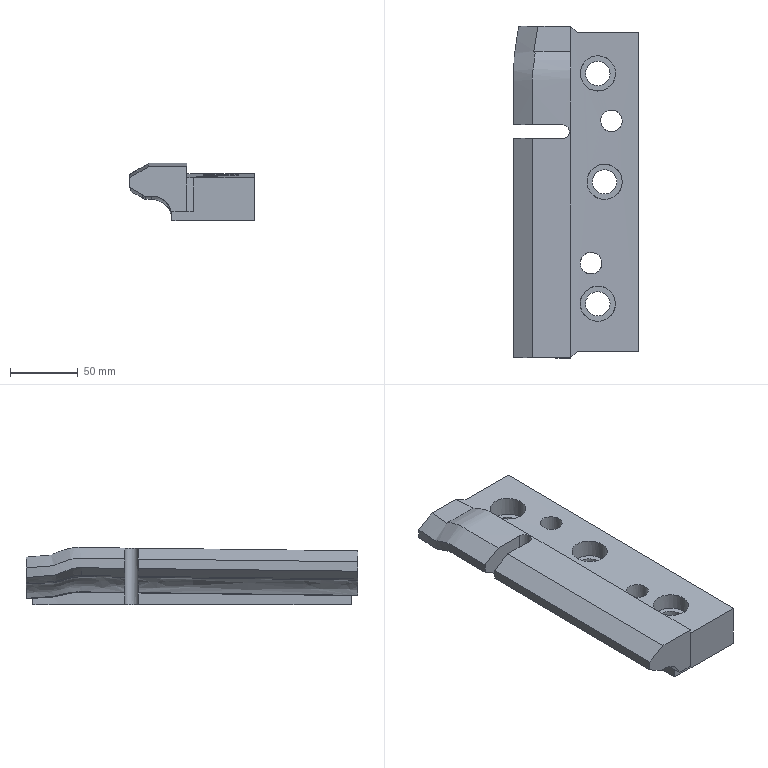Part | NX | features solid 2 | 1 solid | 47 faces | box 92.247 x 245.623 x 42.217 mm | volume 588727 mm3 | spline 22 | plane 16 | cylinder 9 | commonest cylinder face diameters 18 x3 26 x3 16 x2 10 x1